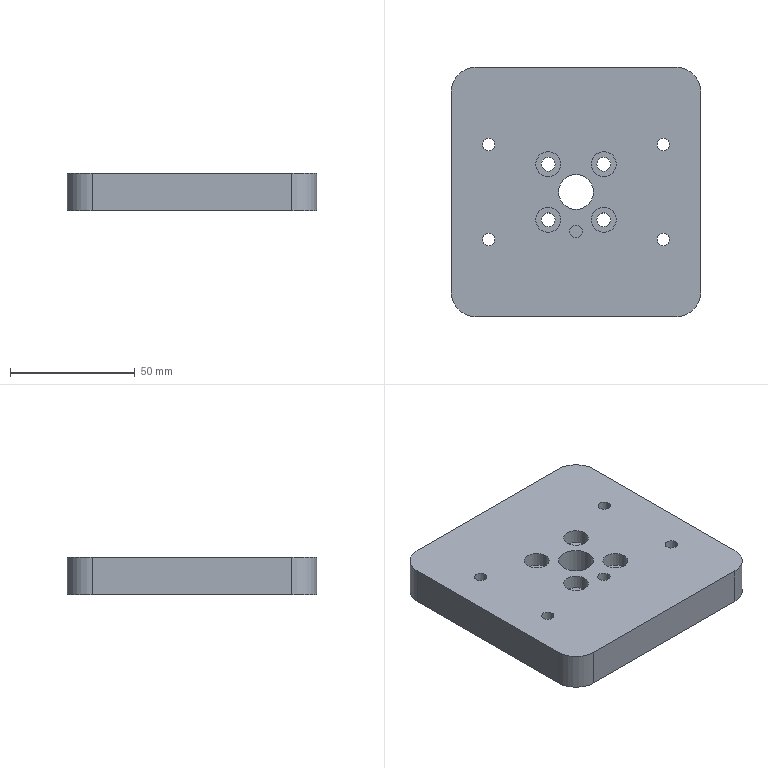NC program | NX | posted with a generic post | part box 100 x 100 x 15 mm
Whole program:
N10 G17 G21 G94 G90
(FLOOR_WALL_1_COPY , TOOL : D63)
N12 T01 M6
N14 G54
N16 G17 G0 G90 X-84.5 Y49.997 S6500 M3
N18 G43 Z30. H1
N20 Z5.
N22 G94 G1 Z2. F1500.
N24 X-81.5
N26 X81.5
N28 Y25.065
N30 X-81.5
N32 Y0.132
N34 X81.5
N36 Y-24.8
N38 X-81.5
N40 X-84.5
N42 Z5.
N44 G0 Z30.
N46 Y49.997
N48 Z4.
N50 G1 Z1.
N52 X-81.5
N54 X81.5
N56 Y25.065
N58 X-81.5
N60 Y0.132
N62 X81.5
N64 Y-24.8
N66 X-81.5
N68 X-84.5
N70 Z4.
N72 G0 Z30.
N74 Y49.997
N76 Z3.
N78 G1 Z0.
N80 X-81.5
N82 X81.5
N84 Y25.065
N86 X-81.5
N88 Y0.132
N90 X81.5
N92 Y-24.8
N94 X-81.5
N96 X-84.5
N98 Z3.
N100 G0 Z30.
N102 M5
(HOLE_MILLING_COPY_1 , TOOL : D10)
N104 T10 M6
N106 G54
N108 G17 G0 G90 X0. Y0. S9500 M3
N110 G43 Z30. H10
N112 Z0.5
N114 G94 G3 X-3.29 Y3.29 R3.29 F2200.
N116 X-6.58 Y0. R3.29
N118 X-6.58 Y0. Z-0.5 I6.58 J0.
N120 X-6.58 Y0. Z-1.5 I6.58 J0.
N122 X-6.58 Y0. Z-2.5 I6.58 J0.
N124 X6.58 Y0. Z-3. I6.58 J0.
N126 X0. Y6.58 R6.58
N128 X6.58 Y0. R-6.58
N130 X3.29 Y3.29 R3.29
N132 X0. Y0. R3.29
N134 G0 Z0.5
N136 G3 X-5.58 Y5.58 R5.58
N138 X-11.16 Y0. R5.58
N140 X-11.16 Y0. Z-0.5 I11.16 J0.
N142 X-11.16 Y0. Z-1.5 I11.16 J0.
N144 X-11.16 Y0. Z-2.5 I11.16 J0.
N146 X11.16 Y0. Z-3. I11.16 J0.
N148 X0. Y11.16 R11.16
N150 X11.16 Y0. R-11.16
N152 X5.58 Y5.58 R5.58
N154 X0. Y0. R5.58
N156 G0 Z0.5
N158 G3 X-7.87 Y7.87 R7.87
N160 X-15.74 Y0. R7.87
N162 X-15.74 Y0. Z-0.5 I15.74 J0.
N164 X-15.74 Y0. Z-1.5 I15.74 J0.
N166 X-15.74 Y0. Z-2.5 I15.74 J0.
N168 X15.74 Y0. Z-3. I15.74 J0.
N170 X0. Y15.74 R15.74
N172 X15.74 Y0. R-15.74
N174 X7.87 Y7.87 R7.87
N176 X0. Y0. R7.87
N178 G0 Z0.5
N180 G3 X-10.16 Y10.16 R10.16
N182 X-20.32 Y0. R10.16
N184 X-20.32 Y0. Z-0.5 I20.32 J0.
N186 X-20.32 Y0. Z-1.5 I20.32 J0.
N188 X-20.32 Y0. Z-2.5 I20.32 J0.
N190 X20.32 Y0. Z-3. I20.32 J0.
N192 X0. Y20.32 R20.32
N194 X20.32 Y0. R-20.32
N196 X10.16 Y10.16 R10.16
N198 X0. Y0. R10.16
N200 G0 Z0.5
N202 G3 X-12.45 Y12.45 R12.45
N204 X-24.9 Y0. R12.45
N206 X-24.9 Y0. Z-0.5 I24.9 J0.
N208 X-24.9 Y0. Z-1.5 I24.9 J0.
N210 X-24.9 Y0. Z-2.5 I24.9 J0.
N212 X24.9 Y0. Z-3. I24.9 J0.
N214 X0. Y24.9 R24.9
N216 X24.9 Y0. R-24.9
N218 X12.45 Y12.45 R12.45
N220 X0. Y0. R12.45
N222 G0 Z30.
N224 M5
(PLANAR_MILL_COPY , TOOL : D6A45)
N226 T07 M6
N228 G54
N230 G17 G0 G90 X-36.1 Y19.866 S9500 M3
N232 G43 Z30. H7
N234 Z0.5
N236 G94 G1 Z-1. F1250.
N238 G3 X-36.6 Y19. R1.
N240 X-35. Y17.4 R1.6
N242 X-36.6 Y19. R-1.6
N244 X-36.1 Y18.134 R1.
N246 G1 Z0.5
N248 G0 Z30.
N250 Y-18.134
N252 Z0.5
N254 G1 Z-1.
N256 G3 X-36.6 Y-19. R1.
N258 X-35. Y-20.6 R1.6
N260 X-36.6 Y-19. R-1.6
N262 X-36.1 Y-19.866 R1.
N264 G1 Z0.5
N266 G0 Z30.
N268 X-51.4 Y-0.866
N270 Z0.5
N272 G1 Z-1.
N274 G3 X-50.9 Y0. R1.
N276 G1 Y40.
N278 G2 X-40. Y50.9 R10.9
N280 G1 X40.
N282 G2 X50.9 Y40. R10.9
N284 G1 Y-40.
N286 G2 X40. Y-50.9 R10.9
N288 G1 X-40.
N290 G2 X-50.9 Y-40. R10.9
N292 G1 Y0.
N294 G3 X-51.4 Y0.866 R1.
N296 G1 Z0.5
N298 G0 Z30.
N300 X-28.6
N302 Z0.5
N304 G1 Z-1.
N306 G3 X-29.1 Y0. R1.
N308 X0. Y-29.1 R29.1
N310 X-29.1 Y0. R-29.1
N312 X-28.6 Y-0.866 R1.
N314 G1 Z0.5
N316 G0 Z30.
N318 X36.1 Y-19.866
N320 Z0.5
N322 G1 Z-1.
N324 G3 X36.6 Y-19. R1.
N326 X35. Y-17.4 R1.6
N328 X36.6 Y-19. R-1.6
N330 X36.1 Y-18.134 R1.
N332 G1 Z0.5
N334 G0 Z30.
N336 Y18.134
N338 Z0.5
N340 G1 Z-1.
N342 G3 X36.6 Y19. R1.
N344 X35. Y20.6 R1.6
N346 X36.6 Y19. R-1.6
N348 X36.1 Y19.866 R1.
N350 G1 Z0.5
N352 G0 Z30.
(PLANAR_MILL_COPY_COPY , TOOL : D6A45)
N354 X-9.787 Y-12.003
N356 Z-2.5
N358 G1 Z-4.
N360 G3 X-9.287 Y-11.137 R1.
N362 X-11.137 Y-9.287 R1.85
N364 X-9.287 Y-11.137 R-1.85
N366 X-9.787 Y-10.271 R1.
N368 G1 Z-2.5
N370 G0 Z30.
N372 Y10.271
N374 Z-2.5
N376 G1 Z-4.
N378 G3 X-9.287 Y11.137 R1.
N380 X-11.137 Y12.987 R1.85
N382 X-9.287 Y11.137 R-1.85
N384 X-9.787 Y12.003 R1.
N386 G1 Z-2.5
N388 G0 Z30.
N390 X12.487 Y10.271
N392 Z-2.5
N394 G1 Z-4.
N396 G3 X12.987 Y11.137 R1.
N398 X11.137 Y12.987 R1.85
N400 X12.987 Y11.137 R-1.85
N402 X12.487 Y12.003 R1.
N404 G1 Z-2.5
N406 G0 Z30.
N408 X5.6 Y-0.866
N410 Z-2.5
N412 G1 Z-4.
N414 G3 X6.1 Y0. R1.
N416 X0. Y6.1 R6.1
N418 X6.1 Y0. R-6.1
N420 X5.6 Y0.866 R1.
N422 G1 Z-2.5
N424 G0 Z30.
N426 X12.487 Y-12.003
N428 Z-2.5
N430 G1 Z-4.
N432 G3 X12.987 Y-11.137 R1.
N434 X11.137 Y-9.287 R1.85
N436 X12.987 Y-11.137 R-1.85
N438 X12.487 Y-10.271 R1.
N440 G1 Z-2.5
N442 G0 Z30.
N444 M5
(刀补10 , TOOL : D10)
N446 T10 M6
N448 G54
N450 G17 G0 G90 X-21.539 Y3.362 S9500 M3
N452 G43 Z30. H10
N454 Z0.5
N456 G41 G94 G1 X-21.638 Y3.378 F1200. D10
N458 G3 X-24.95 Y0. R3.379
N460 X-24.95 Y0. Z-2.5 I24.95 J0.
N462 X-12.475 Y-21.607 Z-3. R24.95
N464 X21.607 Y-12.475 R24.95
N466 X-12.475 Y-21.607 R-24.95
N468 X-7.894 Y-20.428 R3.379
N470 G40
N472 G1 X-7.858 Y-20.335
N474 G0 Z30.
N476 M5
N478 M2